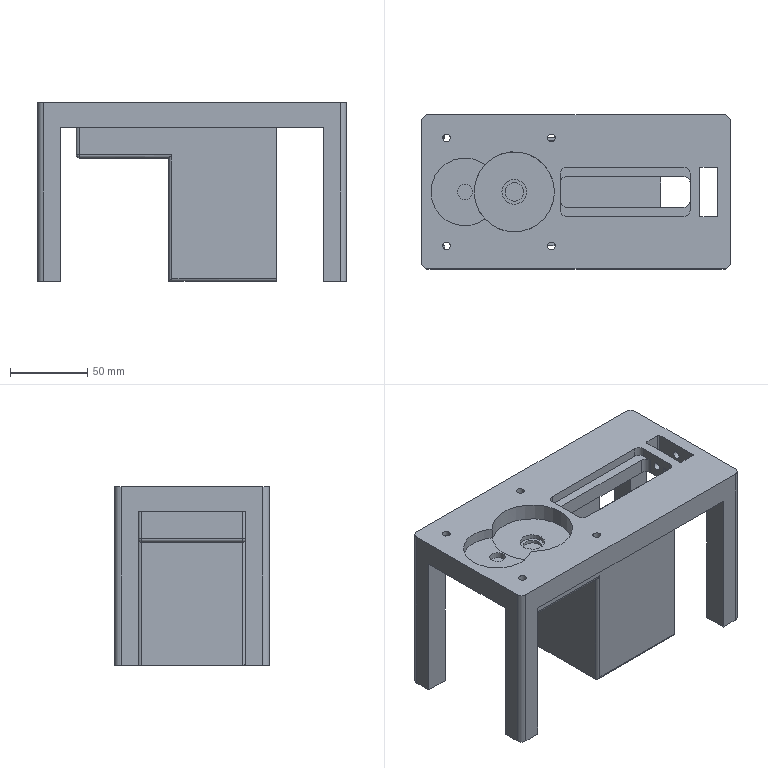Part | NX | features EXTRUDE 14, DATUM_CSYS 8, SKETCH 7, BLEND 4, BREP 1, SHELL 1, UNITE 1 | 1 solid | 101 faces | box 200 x 100 x 116 mm | volume 451086 mm3 | plane 57 | cylinder 40 | sphere 2 | cone 2 | commonest cylinder face diameters 8 x12 4 x9 2 x6 5 x6 4.2 x2 10 x1